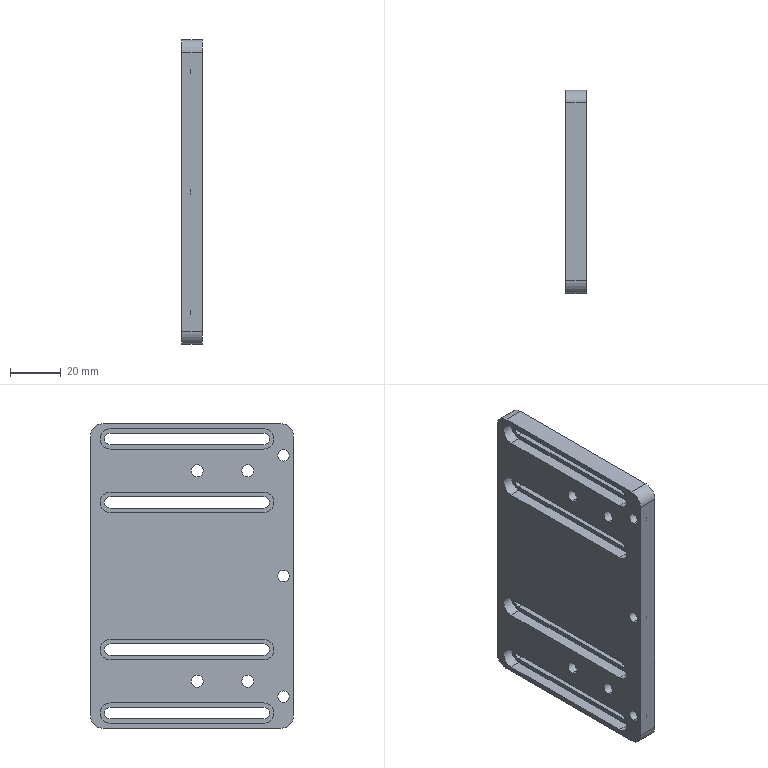Part | SolidWorks | features HoleWzd 3, Extrusion 1, Fillet 1, MirrorPattern 1 | 1 solid | 81 faces | box 8 x 80 x 120 mm | volume 61128 mm3 | cylinder 48 | plane 33 | commonest cylinder face diameters 8 x16 4.5 x14 4.8 x8 7.8 x6 10 x4